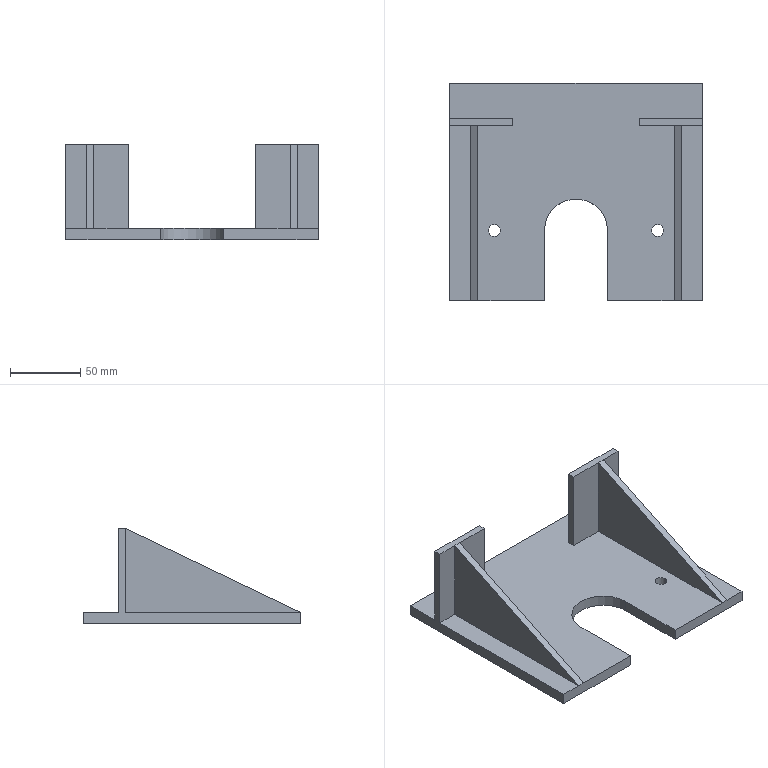Part | STEP file | 1 solid | 32 faces | box 180 x 155 x 68 mm | volume 262430 mm3 | plane 27 | cylinder 5 | commonest cylinder face diameters 8.5 x4 45 x1